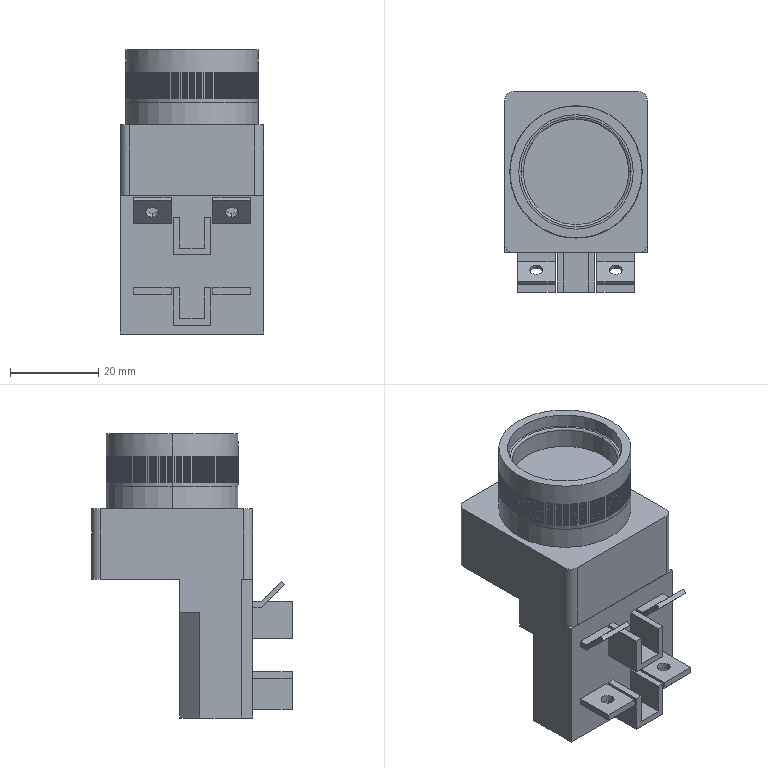Part | STEP file | HANYOUNG CR-253 5A | 4 solids | 1000 faces | box 32.5 x 45.5 x 64.5 mm | volume 42497 mm3 | plane 972 | cylinder 26 | torus 2 | commonest cylinder face diameters 3 x12 4 x4 30 x4 6.718 x2 24 x2 26 x2